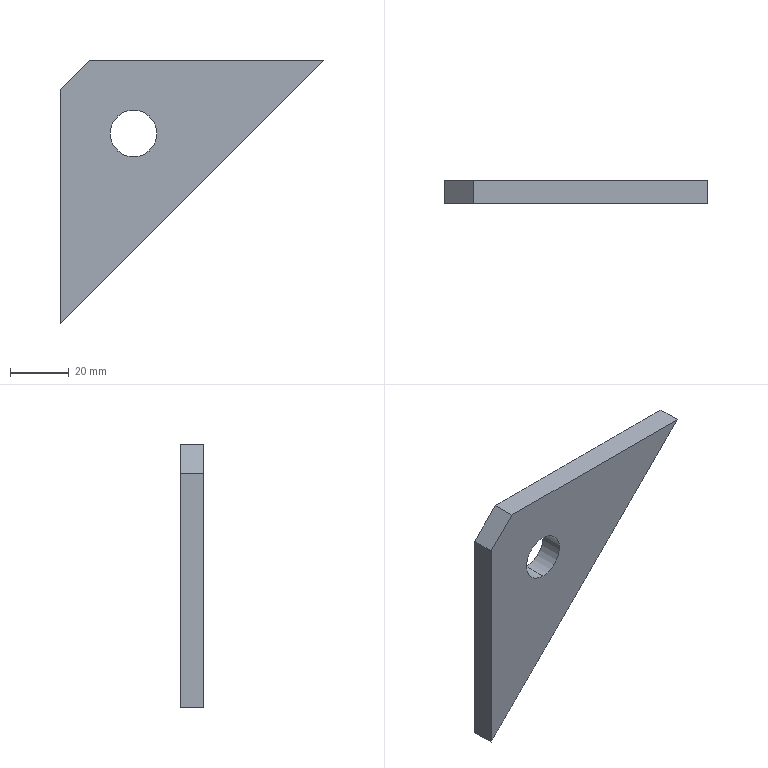Part | SolidWorks | features Chamfer 1, Extrusion 1, HoleWzd 1 | 1 solid | 8 faces | box 90 x 8 x 90 mm | volume 30392 mm3 | plane 6 | cylinder 2 | commonest cylinder face diameters 16 x2
STEP:
#1=CARTESIAN_POINT('',(25.,0.,-33.));
#2=VERTEX_POINT('',#1);
#3=CARTESIAN_POINT('',(25.,0.,-17.));
#4=VERTEX_POINT('',#3);
#5=CARTESIAN_POINT('',(25.,0.,-25.));
#6=DIRECTION('',(0.,1.,0.));
#7=DIRECTION('',(0.,0.,1.));
#8=AXIS2_PLACEMENT_3D('',#5,#6,#7);
#9=CIRCLE('',#8,8.);
#10=EDGE_CURVE('',#2,#4,#9,.T.);
#11=ORIENTED_EDGE('',*,*,#10,.F.);
#12=CARTESIAN_POINT('',(25.,8.,-33.));
#13=VERTEX_POINT('',#12);
#14=CARTESIAN_POINT('',(25.,8.,-33.));
#15=DIRECTION('',(0.,1.,0.));
#16=VECTOR('',#15,1000.);
#17=LINE('',#14,#16);
#18=EDGE_CURVE('',#2,#13,#17,.T.);
#19=ORIENTED_EDGE('',*,*,#18,.T.);
#20=CARTESIAN_POINT('',(25.,8.,-17.));
#21=VERTEX_POINT('',#20);
#22=CARTESIAN_POINT('',(25.,8.,-25.));
#23=DIRECTION('',(0.,1.,0.));
#24=DIRECTION('',(0.,0.,1.));
#25=AXIS2_PLACEMENT_3D('',#22,#23,#24);
#26=CIRCLE('',#25,8.);
#27=EDGE_CURVE('',#13,#21,#26,.T.);
#28=ORIENTED_EDGE('',*,*,#27,.T.);
#29=CARTESIAN_POINT('',(25.,8.,-17.));
#30=DIRECTION('',(0.,1.,0.));
#31=VECTOR('',#30,1000.);
#32=LINE('',#29,#31);
#33=EDGE_CURVE('',#4,#21,#32,.T.);
#34=ORIENTED_EDGE('',*,*,#33,.F.);
#35=EDGE_LOOP('',(#11,#19,#28,#34));
#36=FACE_OUTER_BOUND('',#35,.T.);
#37=CARTESIAN_POINT('',(25.,8.,-25.));
#38=DIRECTION('',(0.,1.,0.));
#39=DIRECTION('',(0.,0.,1.));
#40=AXIS2_PLACEMENT_3D('',#37,#38,#39);
#41=CYLINDRICAL_SURFACE('',#40,8.);
#42=ADVANCED_FACE('',(#36),#41,.F.);
#43=CARTESIAN_POINT('',(10.,8.,0.));
#44=VERTEX_POINT('',#43);
#45=CARTESIAN_POINT('',(90.,8.,0.));
#46=VERTEX_POINT('',#45);
#47=CARTESIAN_POINT('',(90.,8.,0.));
#48=DIRECTION('',(1.,0.,0.));
#49=VECTOR('',#48,1000.);
#50=LINE('',#47,#49);
#51=EDGE_CURVE('',#44,#46,#50,.T.);
#52=ORIENTED_EDGE('',*,*,#51,.F.);
#53=CARTESIAN_POINT('',(10.,0.,0.));
#54=VERTEX_POINT('',#53);
#55=CARTESIAN_POINT('',(10.,8.,0.));
#56=DIRECTION('',(0.,-1.,0.));
#57=VECTOR('',#56,1000.);
#58=LINE('',#55,#57);
#59=EDGE_CURVE('',#44,#54,#58,.T.);
#60=ORIENTED_EDGE('',*,*,#59,.T.);
#61=CARTESIAN_POINT('',(90.,0.,0.));
#62=VERTEX_POINT('',#61);
#63=CARTESIAN_POINT('',(90.,0.,0.));
#64=DIRECTION('',(1.,0.,0.));
#65=VECTOR('',#64,1000.);
#66=LINE('',#63,#65);
#67=EDGE_CURVE('',#54,#62,#66,.T.);
#68=ORIENTED_EDGE('',*,*,#67,.T.);
#69=CARTESIAN_POINT('',(90.,8.,0.));
#70=DIRECTION('',(0.,-1.,0.));
#71=VECTOR('',#70,1000.);
#72=LINE('',#69,#71);
#73=EDGE_CURVE('',#46,#62,#72,.T.);
#74=ORIENTED_EDGE('',*,*,#73,.F.);
#75=EDGE_LOOP('',(#52,#60,#68,#74));
#76=FACE_OUTER_BOUND('',#75,.T.);
#77=CARTESIAN_POINT('',(90.,8.,0.));
#78=DIRECTION('',(0.,0.,-1.));
#79=DIRECTION('',(-1.,0.,0.));
#80=AXIS2_PLACEMENT_3D('',#77,#78,#79);
#81=PLANE('',#80);
#82=ADVANCED_FACE('',(#76),#81,.F.);
#83=CARTESIAN_POINT('',(0.,0.,-90.));
#84=VERTEX_POINT('',#83);
#85=CARTESIAN_POINT('',(0.,0.,-90.));
#86=DIRECTION('',(-0.7071,0.,-0.7071));
#87=VECTOR('',#86,1000.);
#88=LINE('',#85,#87);
#89=EDGE_CURVE('',#62,#84,#88,.T.);
#90=ORIENTED_EDGE('',*,*,#89,.T.);
#91=CARTESIAN_POINT('',(0.,8.,-90.));
#92=VERTEX_POINT('',#91);
#93=CARTESIAN_POINT('',(0.,8.,-90.));
#94=DIRECTION('',(0.,-1.,0.));
#95=VECTOR('',#94,1000.);
#96=LINE('',#93,#95);
#97=EDGE_CURVE('',#92,#84,#96,.T.);
#98=ORIENTED_EDGE('',*,*,#97,.F.);
#99=CARTESIAN_POINT('',(0.,8.,-90.));
#100=DIRECTION('',(-0.7071,0.,-0.7071));
#101=VECTOR('',#100,1000.);
#102=LINE('',#99,#101);
#103=EDGE_CURVE('',#46,#92,#102,.T.);
#104=ORIENTED_EDGE('',*,*,#103,.F.);
#105=ORIENTED_EDGE('',*,*,#73,.T.);
#106=EDGE_LOOP('',(#90,#98,#104,#105));
#107=FACE_OUTER_BOUND('',#106,.T.);
#108=CARTESIAN_POINT('',(0.,8.,-90.));
#109=DIRECTION('',(-0.7071,0.,0.7071));
#110=DIRECTION('',(0.7071,0.,0.7071));
#111=AXIS2_PLACEMENT_3D('',#108,#109,#110);
#112=PLANE('',#111);
#113=ADVANCED_FACE('',(#107),#112,.F.);
#114=CARTESIAN_POINT('',(0.,0.,-10.));
#115=VERTEX_POINT('',#114);
#116=CARTESIAN_POINT('',(0.,0.,0.));
#117=DIRECTION('',(0.,0.,1.));
#118=VECTOR('',#117,1000.);
#119=LINE('',#116,#118);
#120=EDGE_CURVE('',#84,#115,#119,.T.);
#121=ORIENTED_EDGE('',*,*,#120,.T.);
#122=CARTESIAN_POINT('',(0.,8.,-10.));
#123=VERTEX_POINT('',#122);
#124=CARTESIAN_POINT('',(0.,8.,-10.));
#125=DIRECTION('',(0.,1.,0.));
#126=VECTOR('',#125,1000.);
#127=LINE('',#124,#126);
#128=EDGE_CURVE('',#115,#123,#127,.T.);
#129=ORIENTED_EDGE('',*,*,#128,.T.);
#130=CARTESIAN_POINT('',(0.,8.,0.));
#131=DIRECTION('',(0.,0.,1.));
#132=VECTOR('',#131,1000.);
#133=LINE('',#130,#132);
#134=EDGE_CURVE('',#92,#123,#133,.T.);
#135=ORIENTED_EDGE('',*,*,#134,.F.);
#136=ORIENTED_EDGE('',*,*,#97,.T.);
#137=EDGE_LOOP('',(#121,#129,#135,#136));
#138=FACE_OUTER_BOUND('',#137,.T.);
#139=CARTESIAN_POINT('',(0.,8.,0.));
#140=DIRECTION('',(1.,0.,0.));
#141=DIRECTION('',(0.,0.,-1.));
#142=AXIS2_PLACEMENT_3D('',#139,#140,#141);
#143=PLANE('',#142);
#144=ADVANCED_FACE('',(#138),#143,.F.);
#145=CARTESIAN_POINT('',(25.,8.,-25.));
#146=DIRECTION('',(0.,1.,0.));
#147=DIRECTION('',(0.,0.,1.));
#148=AXIS2_PLACEMENT_3D('',#145,#146,#147);
#149=CIRCLE('',#148,8.);
#150=EDGE_CURVE('',#21,#13,#149,.T.);
#151=ORIENTED_EDGE('',*,*,#150,.F.);
#152=ORIENTED_EDGE('',*,*,#27,.F.);
#153=EDGE_LOOP('',(#151,#152));
#154=FACE_BOUND('',#153,.T.);
#155=ORIENTED_EDGE('',*,*,#134,.T.);
#156=CARTESIAN_POINT('',(10.,8.,0.));
#157=DIRECTION('',(0.7071,0.,0.7071));
#158=VECTOR('',#157,1000.);
#159=LINE('',#156,#158);
#160=EDGE_CURVE('',#123,#44,#159,.T.);
#161=ORIENTED_EDGE('',*,*,#160,.T.);
#162=ORIENTED_EDGE('',*,*,#51,.T.);
#163=ORIENTED_EDGE('',*,*,#103,.T.);
#164=EDGE_LOOP('',(#155,#161,#162,#163));
#165=FACE_OUTER_BOUND('',#164,.T.);
#166=CARTESIAN_POINT('',(0.,8.,0.));
#167=DIRECTION('',(0.,-1.,0.));
#168=DIRECTION('',(0.,0.,-1.));
#169=AXIS2_PLACEMENT_3D('',#166,#167,#168);
#170=PLANE('',#169);
#171=ADVANCED_FACE('',(#154,#165),#170,.F.);
#172=CARTESIAN_POINT('',(25.,0.,-25.));
#173=DIRECTION('',(0.,1.,0.));
#174=DIRECTION('',(0.,0.,1.));
#175=AXIS2_PLACEMENT_3D('',#172,#173,#174);
#176=CIRCLE('',#175,8.);
#177=EDGE_CURVE('',#4,#2,#176,.T.);
#178=ORIENTED_EDGE('',*,*,#177,.T.);
#179=ORIENTED_EDGE('',*,*,#10,.T.);
#180=EDGE_LOOP('',(#178,#179));
#181=FACE_BOUND('',#180,.T.);
#182=ORIENTED_EDGE('',*,*,#67,.F.);
#183=CARTESIAN_POINT('',(5.,0.,-5.));
#184=DIRECTION('',(-0.7071,0.,-0.7071));
#185=VECTOR('',#184,1000.);
#186=LINE('',#183,#185);
#187=EDGE_CURVE('',#54,#115,#186,.T.);
#188=ORIENTED_EDGE('',*,*,#187,.T.);
#189=ORIENTED_EDGE('',*,*,#120,.F.);
#190=ORIENTED_EDGE('',*,*,#89,.F.);
#191=EDGE_LOOP('',(#182,#188,#189,#190));
#192=FACE_OUTER_BOUND('',#191,.T.);
#193=CARTESIAN_POINT('',(0.,0.,0.));
#194=DIRECTION('',(0.,-1.,0.));
#195=DIRECTION('',(0.,0.,-1.));
#196=AXIS2_PLACEMENT_3D('',#193,#194,#195);
#197=PLANE('',#196);
#198=ADVANCED_FACE('',(#181,#192),#197,.T.);
#199=ORIENTED_EDGE('',*,*,#160,.F.);
#200=ORIENTED_EDGE('',*,*,#128,.F.);
#201=ORIENTED_EDGE('',*,*,#187,.F.);
#202=ORIENTED_EDGE('',*,*,#59,.F.);
#203=EDGE_LOOP('',(#199,#200,#201,#202));
#204=FACE_OUTER_BOUND('',#203,.T.);
#205=CARTESIAN_POINT('',(10.,8.,0.));
#206=DIRECTION('',(0.7071,0.,-0.7071));
#207=DIRECTION('',(0.,-1.,0.));
#208=AXIS2_PLACEMENT_3D('',#205,#206,#207);
#209=PLANE('',#208);
#210=ADVANCED_FACE('',(#204),#209,.F.);
#211=ORIENTED_EDGE('',*,*,#18,.F.);
#212=ORIENTED_EDGE('',*,*,#177,.F.);
#213=ORIENTED_EDGE('',*,*,#33,.T.);
#214=ORIENTED_EDGE('',*,*,#150,.T.);
#215=EDGE_LOOP('',(#211,#212,#213,#214));
#216=FACE_OUTER_BOUND('',#215,.T.);
#217=CARTESIAN_POINT('',(25.,8.,-25.));
#218=DIRECTION('',(0.,1.,0.));
#219=DIRECTION('',(0.,0.,1.));
#220=AXIS2_PLACEMENT_3D('',#217,#218,#219);
#221=CYLINDRICAL_SURFACE('',#220,8.);
#222=ADVANCED_FACE('',(#216),#221,.F.);
#223=CLOSED_SHELL('',(#42,#82,#113,#144,#171,#198,#210,#222));
#224=MANIFOLD_SOLID_BREP('',#223);
#225=CARTESIAN_POINT('',(0.,0.,0.));
#226=DIRECTION('',(0.,0.,1.));
#227=DIRECTION('',(1.,0.,0.));
#228=AXIS2_PLACEMENT_3D('',#225,#226,#227);
#229=(LENGTH_UNIT()NAMED_UNIT(*)SI_UNIT(.MILLI.,.METRE.));
#230=UNCERTAINTY_MEASURE_WITH_UNIT(LENGTH_MEASURE(0.00001),#229,'','');
#231=(NAMED_UNIT(*)PLANE_ANGLE_UNIT()SI_UNIT($,.RADIAN.));
#232=(NAMED_UNIT(*)SI_UNIT($,.STERADIAN.)SOLID_ANGLE_UNIT());
#233=(GEOMETRIC_REPRESENTATION_CONTEXT(3)GLOBAL_UNCERTAINTY_ASSIGNED_CONTEXT((#230))GLOBAL_UNIT_ASSIGNED_CONTEXT((#229,#231,#232))REPRESENTATION_CONTEXT('',''));
#234=ADVANCED_BREP_SHAPE_REPRESENTATION('',(#224,#228),#233);